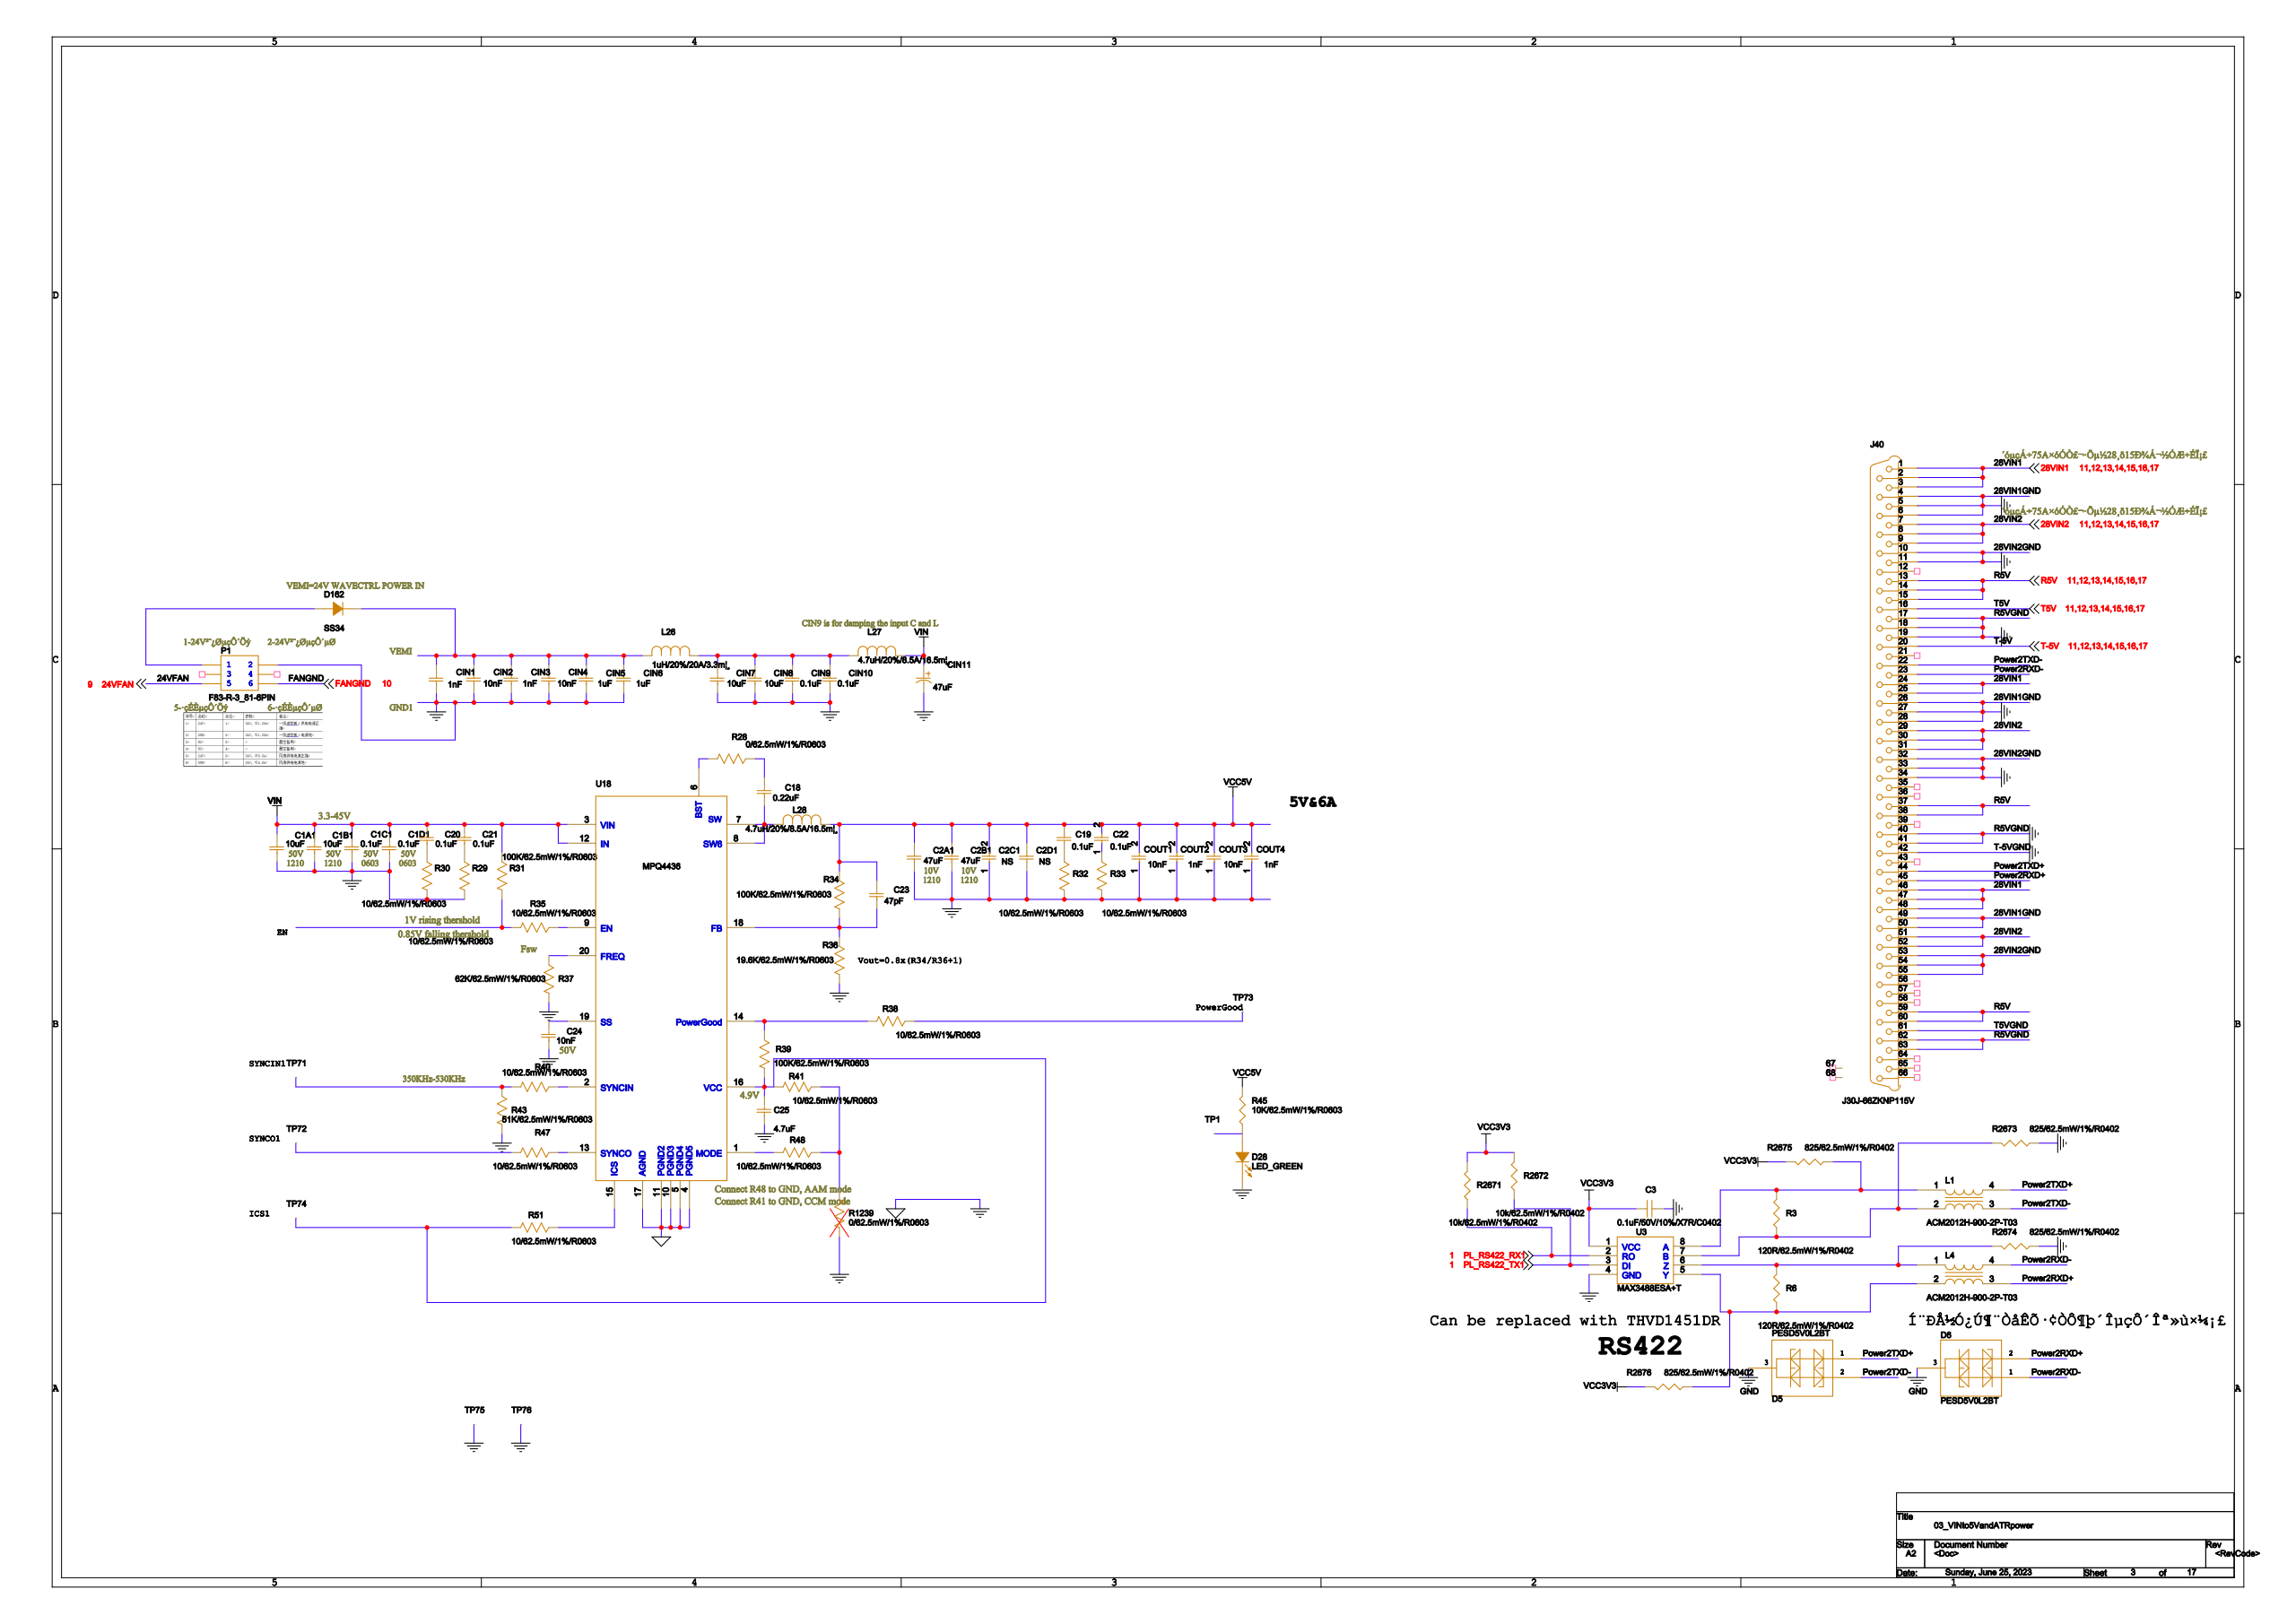Circuit board | Cadence Allegro | 1997 parts | 1536 nets | one sheet of the schematic
Parts on this sheet (reference | value | footprint):
C1A1 | CAP/1210 | 1210
C1B1 | CAP/1210 | 1210
C1C1 | CAP/0603 | 0603C
C1D1 | CAP/0603 | 0603C
C2A1 | CAP/1210 | 1210
C2B1 | CAP/1210 | 1210
C2C1 | CAP/0603 | 0603C
C2D1 | CAP/0603 | 0603C
C3 | 0.1uF/50V/10%/X7R/C0402 | 0402
C18 | CAP/0603 | 0603C
C19 | CAP/0603 | 0603C
C20 | CAP/0603 | 0603C
C21 | CAP/0603 | 0603C
C22 | CAP/0603 | 0603C
C23 | CAP/0603 | 0603C
C24 | CAP/0603 | 0603C
C25 | CAP/0603 | 0603C
CIN1 | CAP/0603 | 0603C
CIN2 | CAP/0603 | 0603C
CIN3 | CAP/0603 | 0603C
CIN4 | CAP/0603 | 0603C
CIN5 | CAP/0603 | 0805C
CIN6 | CAP/0603 | 0805C
CIN7 | CAP/0603 | 1206
CIN8 | CAP/0603 | 1206
CIN9 | CAP/0603 | 0603C
CIN10 | CAP/0603 | 0603C
CIN11 | CAP/ELECT/DIP/OD5.3P2.0 | AP-SMD_BD6_3-L6_6-W6_6-LS7_21
COUT1 | CAP/0603 | 0603C
COUT2 | CAP/0603 | 0603C
COUT3 | CAP/0603 | 0603C
COUT4 | CAP/0603 | 0603C
D5 | PESD5V0L2BT | SOT23
D6 | PESD5V0L2BT | SOT23
D28 | LED_GREEN | LED0805
D162 | SS34 | DO-214AC
J40 | J30J-66ZKNP115V | J30J-66ZKNP115V
L1 | ACM2012H-900-2P-T03 | ACM2012
L4 | ACM2012H-900-2P-T03 | ACM2012
L26 | CKST1004-1uH/M-B | SMD_10X11
L27 | CKST1004-4.7uH/M | SMD_10X11
L28 | CKST1004-4.7uH/M | SMD_10X11
P1 | F83-R-3_81-6PIN | F83-R-3_81-6PIN
R3 | 120R/62.5mW/1%/R0402 | 0402
R6 | 120R/62.5mW/1%/R0402 | 0402
R28 | 0/62.5mW/1%/R0603 | 0603R
R29 | 10/62.5mW/1%/R0603 | 0603R
R30 | 10/62.5mW/1%/R0603 | 0603R
R31 | 100K/62.5mW/1%/R0603 | 0603R
R32 | 10/62.5mW/1%/R0603 | 0603R
R33 | 10/62.5mW/1%/R0603 | 0603R
R34 | 100K/62.5mW/1%/R0603 | 0603R
R35 | 10/62.5mW/1%/R0603 | 0603R
R36 | 19.6K/62.5mW/1%/R0603 | 0603R
R37 | 62K/62.5mW/1%/R0603 | 0603R
R38 | 10/62.5mW/1%/R0603 | 0603R
R39 | 100K/62.5mW/1%/R0603 | 0603R
R40 | 10/62.5mW/1%/R0603 | 0603R
R41 | 10/62.5mW/1%/R0603 | 0603R
R43 | 51K/62.5mW/1%/R0603 | 0603R
R45 | 10K/62.5mW/1%/R0603 | 0603R
R47 | 10/62.5mW/1%/R0603 | 0603R
R48 | 10/62.5mW/1%/R0603 | 0603R
R51 | 10/62.5mW/1%/R0603 | 0603R
R1239 | 0/62.5mW/1%/R0603 | 0603R
R2671 | 10K/62.5mW/1%/R0402 | 0402
R2672 | 10K/62.5mW/1%/R0402 | 0402
R2673 | 825/62.5mW/1%/R0402 | 0402
R2674 | 825/62.5mW/1%/R0402 | 0402
R2675 | 825/62.5mW/1%/R0402 | 0402
R2676 | 825/62.5mW/1%/R0402 | 0402
TP1 | TEST POINT A | TEST_12MM
TP71 | TEST POINT A | TEST_12MM
TP72 | TEST POINT A | TEST_12MM
TP73 | TEST POINT A | TEST_12MM
TP74 | TEST POINT A | TEST_12MM
TP75 | TEST POINT A | TEST_1MM
TP76 | TEST POINT A | TEST_1MM
U3 | MAX3488ESA+T | SO8
U18 | MPQ4436 | QFN-4X4_MPQ4436-AEC1_MNP
Nets of these parts (net: part-pin ...):
3.3V: C3-1 R2671-1 R2672-1 R2675-1 R2676-1 U3-1
AGND: C1A1-2 C1B1-2 C1C1-2 C1D1-2 C2A1-2 C2B1-2 C2C1-1 C2D1-1 C3-2 C24-2 C25-2 CIN1-2 CIN2-2 CIN3-2 CIN4-2 CIN5-2 CIN6-2 CIN7-2 CIN8-2 CIN9-2 CIN10-2 CIN11-2 COUT1-1 COUT2-1 COUT3-1 COUT4-1 D5-3 D6-3 D28-2 P1-2 R29-2 R30-2 R32-2 R33-2 R36-1 R37-2 R43-1 R1239-2 R2673-2 R2674-2 TP75-1 TP76-1 U3-4 U18-4 U18-5 U18-10 U18-11 U18-17 J40-4 J40-5 J40-6 J40-10 J40-11 J40-17 J40-18 J40-19 J40-26 J40-27 J40-28 J40-32 J40-33 J40-34 J40-40 J40-41 J40-42 J40-49 J40-50 J40-53 J40-54 J40-55 J40-62 J40-63
N23886899: L1-2 R3-2 R2673-1 U3-7
N23886907: L4-1 R6-1 R2674-1 U3-6
N23886887: L1-1 R3-1 R2675-2 U3-8
N23886911: L4-2 R6-2 R2676-2 U3-5
PL_RS422_RX1: R2671-2 U3-2
PL_RS422_TX1: R2672-2 U3-3
VCC5V: C2A1-1 C2B1-1 C2C1-2 C2D1-2 C19-2 C22-2 C23-1 COUT1-2 COUT2-2 COUT3-2 COUT4-2 L28-2 R34-2 R45-2
FANGND: P1-6
N23492270: D162-1 P1-1
24VFAN: P1-5
R5V: J40-13 J40-14 J40-15 J40-16 J40-37 J40-38 J40-59 J40-60
28VIN1: J40-1 J40-2 J40-3 J40-24 J40-25 J40-46 J40-47 J40-48
T-5V: J40-20
POWER2TXD-: D5-2 L1-3 J40-22
POWER2RXD-: D6-1 L4-4 J40-23
28VIN2: J40-7 J40-8 J40-9 J40-29 J40-30 J40-31 J40-51 J40-52
POWER2TXD+: D5-1 L1-4 J40-44
POWER2RXD+: D6-2 L4-3 J40-45
T5VGND: J40-61
N23491928: CIN1-1 CIN2-1 CIN3-1 CIN4-1 CIN5-1 CIN6-1 D162-2 L26-1
N23492006: R28-1 U18-6
N23491998: R35-2 U18-9
N23492020: C23-2 R34-1 R36-2 U18-18
N23491924: R37-1 U18-20
N23491980: R51-1 U18-15
VIN: C1A1-1 C1B1-1 C1C1-1 C1D1-1 C20-1 C21-1 CIN11-1 L27-2 R31-2 U18-3 U18-12
N23491986: R48-2 U18-1
N23491988: R38-2 R39-2 U18-14
N23491922: C24-1 U18-19
N23492014: C18-2 L28-1 U18-7 U18-8
N23491926: R40-2 U18-2
N23491976: R47-2 U18-13
N23491984: C25-1 R39-1 R41-2 R51-2 TP74-1 U18-16
N23492010: C18-1 R28-2
N234914480: C19-1 R32-1
N234914160: C20-2 R30-1
N234916911: C21-2 R29-1
N23492183: C22-1 R33-1
N23491954: CIN7-1 CIN8-1 CIN9-1 CIN10-1 L26-2 L27-1
N23491994: R41-1 R48-1 R1239-1
N23492000: R31-1 R35-1
N23492076: R38-1 TP73-1
N23491972: R40-1 R43-2 TP71-1
N23492221: D28-1 R45-1 TP1-1
N23491978: R47-1 TP72-1